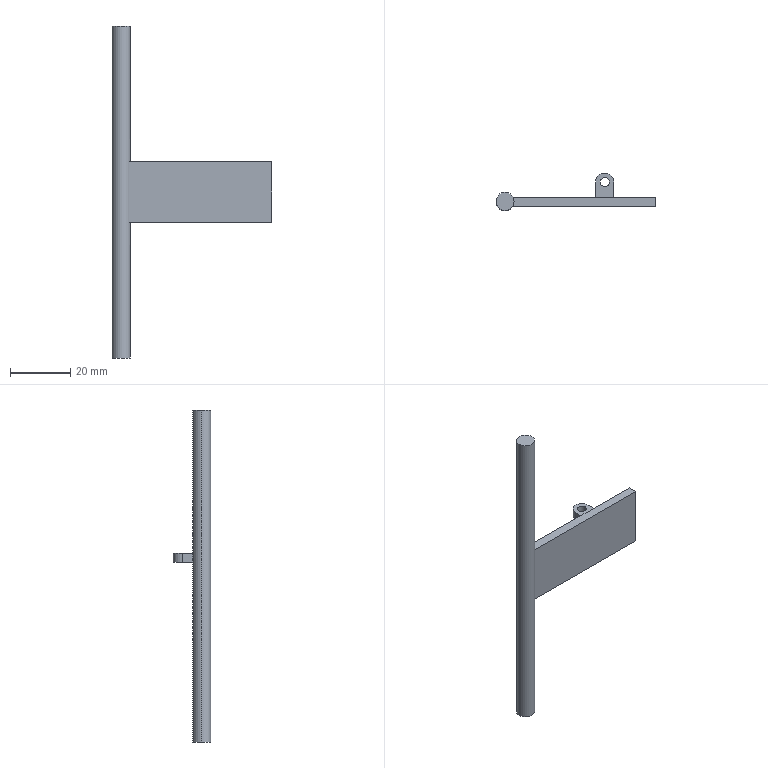Part | SolidWorks | features ICE 2, Extrusion 1 | 1 solid | 16 faces | box 53 x 12.5 x 110 mm | volume 6049 mm3 | plane 11 | cylinder 5 | commonest cylinder face diameters 6 x3 3 x2
STEP:
#1=CARTESIAN_POINT('',(31.5,6.5,4.5));
#2=VERTEX_POINT('',#1);
#3=CARTESIAN_POINT('',(34.5,6.5,4.5));
#4=VERTEX_POINT('',#3);
#5=CARTESIAN_POINT('',(33.,6.5,4.5));
#6=DIRECTION('',(0.,0.,1.));
#7=DIRECTION('',(1.,0.,0.));
#8=AXIS2_PLACEMENT_3D('',#5,#6,#7);
#9=CIRCLE('',#8,1.5);
#10=EDGE_CURVE('',#2,#4,#9,.T.);
#11=ORIENTED_EDGE('',*,*,#10,.F.);
#12=CARTESIAN_POINT('',(31.5,6.5,7.5));
#13=VERTEX_POINT('',#12);
#14=CARTESIAN_POINT('',(31.5,6.5,4.5));
#15=DIRECTION('',(0.,0.,1.));
#16=VECTOR('',#15,1000.);
#17=LINE('',#14,#16);
#18=EDGE_CURVE('',#2,#13,#17,.T.);
#19=ORIENTED_EDGE('',*,*,#18,.T.);
#20=CARTESIAN_POINT('',(34.5,6.5,7.5));
#21=VERTEX_POINT('',#20);
#22=CARTESIAN_POINT('',(33.,6.5,7.5));
#23=DIRECTION('',(0.,0.,1.));
#24=DIRECTION('',(1.,0.,0.));
#25=AXIS2_PLACEMENT_3D('',#22,#23,#24);
#26=CIRCLE('',#25,1.5);
#27=EDGE_CURVE('',#13,#21,#26,.T.);
#28=ORIENTED_EDGE('',*,*,#27,.T.);
#29=CARTESIAN_POINT('',(34.5,6.5,4.5));
#30=DIRECTION('',(0.,0.,1.));
#31=VECTOR('',#30,1000.);
#32=LINE('',#29,#31);
#33=EDGE_CURVE('',#4,#21,#32,.T.);
#34=ORIENTED_EDGE('',*,*,#33,.F.);
#35=EDGE_LOOP('',(#11,#19,#28,#34));
#36=FACE_OUTER_BOUND('',#35,.T.);
#37=CARTESIAN_POINT('',(33.,6.5,4.5));
#38=DIRECTION('',(0.,0.,1.));
#39=DIRECTION('',(1.,0.,0.));
#40=AXIS2_PLACEMENT_3D('',#37,#38,#39);
#41=CYLINDRICAL_SURFACE('',#40,1.5);
#42=ADVANCED_FACE('',(#36),#41,.F.);
#43=CARTESIAN_POINT('',(3.,0.,55.));
#44=VERTEX_POINT('',#43);
#45=CARTESIAN_POINT('',(-3.,0.,55.));
#46=VERTEX_POINT('',#45);
#47=CARTESIAN_POINT('',(0.,0.,55.));
#48=DIRECTION('',(0.,0.,1.));
#49=DIRECTION('',(1.,0.,0.));
#50=AXIS2_PLACEMENT_3D('',#47,#48,#49);
#51=CIRCLE('',#50,3.);
#52=EDGE_CURVE('',#44,#46,#51,.T.);
#53=ORIENTED_EDGE('',*,*,#52,.F.);
#54=CARTESIAN_POINT('',(3.,0.,10.));
#55=VERTEX_POINT('',#54);
#56=CARTESIAN_POINT('',(3.,0.,55.));
#57=DIRECTION('',(0.,0.,-1.));
#58=VECTOR('',#57,1000.);
#59=LINE('',#56,#58);
#60=EDGE_CURVE('',#44,#55,#59,.T.);
#61=ORIENTED_EDGE('',*,*,#60,.T.);
#62=CARTESIAN_POINT('',(2.598,1.5,10.));
#63=VERTEX_POINT('',#62);
#64=CARTESIAN_POINT('',(0.,0.,10.));
#65=DIRECTION('',(0.,0.,-1.));
#66=DIRECTION('',(-1.,0.,0.));
#67=AXIS2_PLACEMENT_3D('',#64,#65,#66);
#68=CIRCLE('',#67,3.);
#69=EDGE_CURVE('',#63,#55,#68,.T.);
#70=ORIENTED_EDGE('',*,*,#69,.F.);
#71=CARTESIAN_POINT('',(2.598,1.5,-10.));
#72=VERTEX_POINT('',#71);
#73=CARTESIAN_POINT('',(2.598,1.5,55.));
#74=DIRECTION('',(0.,0.,1.));
#75=VECTOR('',#74,1000.);
#76=LINE('',#73,#75);
#77=EDGE_CURVE('',#72,#63,#76,.T.);
#78=ORIENTED_EDGE('',*,*,#77,.F.);
#79=CARTESIAN_POINT('',(3.,0.,-10.));
#80=VERTEX_POINT('',#79);
#81=CARTESIAN_POINT('',(0.,0.,-10.));
#82=DIRECTION('',(0.,0.,-1.));
#83=DIRECTION('',(-1.,0.,0.));
#84=AXIS2_PLACEMENT_3D('',#81,#82,#83);
#85=CIRCLE('',#84,3.);
#86=EDGE_CURVE('',#72,#80,#85,.T.);
#87=ORIENTED_EDGE('',*,*,#86,.T.);
#88=CARTESIAN_POINT('',(3.,0.,-55.));
#89=VERTEX_POINT('',#88);
#90=CARTESIAN_POINT('',(3.,0.,55.));
#91=DIRECTION('',(0.,0.,-1.));
#92=VECTOR('',#91,1000.);
#93=LINE('',#90,#92);
#94=EDGE_CURVE('',#80,#89,#93,.T.);
#95=ORIENTED_EDGE('',*,*,#94,.T.);
#96=CARTESIAN_POINT('',(-3.,0.,-55.));
#97=VERTEX_POINT('',#96);
#98=CARTESIAN_POINT('',(0.,0.,-55.));
#99=DIRECTION('',(0.,0.,1.));
#100=DIRECTION('',(1.,0.,0.));
#101=AXIS2_PLACEMENT_3D('',#98,#99,#100);
#102=CIRCLE('',#101,3.);
#103=EDGE_CURVE('',#89,#97,#102,.T.);
#104=ORIENTED_EDGE('',*,*,#103,.T.);
#105=CARTESIAN_POINT('',(-3.,0.,55.));
#106=DIRECTION('',(0.,0.,-1.));
#107=VECTOR('',#106,1000.);
#108=LINE('',#105,#107);
#109=EDGE_CURVE('',#46,#97,#108,.T.);
#110=ORIENTED_EDGE('',*,*,#109,.F.);
#111=EDGE_LOOP('',(#53,#61,#70,#78,#87,#95,#104,#110));
#112=FACE_OUTER_BOUND('',#111,.T.);
#113=CARTESIAN_POINT('',(0.,0.,55.));
#114=DIRECTION('',(0.,0.,-1.));
#115=DIRECTION('',(-1.,0.,0.));
#116=AXIS2_PLACEMENT_3D('',#113,#114,#115);
#117=CYLINDRICAL_SURFACE('',#116,3.);
#118=ADVANCED_FACE('',(#112),#117,.T.);
#119=CARTESIAN_POINT('',(50.,1.5,-10.));
#120=VERTEX_POINT('',#119);
#121=CARTESIAN_POINT('',(50.,1.5,-10.));
#122=DIRECTION('',(-1.,0.,0.));
#123=VECTOR('',#122,1000.);
#124=LINE('',#121,#123);
#125=EDGE_CURVE('',#120,#72,#124,.T.);
#126=ORIENTED_EDGE('',*,*,#125,.T.);
#127=ORIENTED_EDGE('',*,*,#77,.T.);
#128=CARTESIAN_POINT('',(50.,1.5,10.));
#129=VERTEX_POINT('',#128);
#130=CARTESIAN_POINT('',(50.,1.5,10.));
#131=DIRECTION('',(-1.,0.,0.));
#132=VECTOR('',#131,1000.);
#133=LINE('',#130,#132);
#134=EDGE_CURVE('',#129,#63,#133,.T.);
#135=ORIENTED_EDGE('',*,*,#134,.F.);
#136=CARTESIAN_POINT('',(50.,1.5,10.));
#137=DIRECTION('',(0.,0.,-1.));
#138=VECTOR('',#137,1000.);
#139=LINE('',#136,#138);
#140=EDGE_CURVE('',#129,#120,#139,.T.);
#141=ORIENTED_EDGE('',*,*,#140,.T.);
#142=EDGE_LOOP('',(#126,#127,#135,#141));
#143=FACE_OUTER_BOUND('',#142,.T.);
#144=CARTESIAN_POINT('',(30.,1.5,4.5));
#145=VERTEX_POINT('',#144);
#146=CARTESIAN_POINT('',(36.,1.5,4.5));
#147=VERTEX_POINT('',#146);
#148=CARTESIAN_POINT('',(0.,1.5,4.5));
#149=DIRECTION('',(1.,0.,0.));
#150=VECTOR('',#149,1000.);
#151=LINE('',#148,#150);
#152=EDGE_CURVE('',#145,#147,#151,.T.);
#153=ORIENTED_EDGE('',*,*,#152,.T.);
#154=CARTESIAN_POINT('',(36.,1.5,7.5));
#155=VERTEX_POINT('',#154);
#156=CARTESIAN_POINT('',(36.,1.5,4.5));
#157=DIRECTION('',(0.,0.,1.));
#158=VECTOR('',#157,1000.);
#159=LINE('',#156,#158);
#160=EDGE_CURVE('',#147,#155,#159,.T.);
#161=ORIENTED_EDGE('',*,*,#160,.T.);
#162=CARTESIAN_POINT('',(30.,1.5,7.5));
#163=VERTEX_POINT('',#162);
#164=CARTESIAN_POINT('',(0.,1.5,7.5));
#165=DIRECTION('',(1.,0.,0.));
#166=VECTOR('',#165,1000.);
#167=LINE('',#164,#166);
#168=EDGE_CURVE('',#163,#155,#167,.T.);
#169=ORIENTED_EDGE('',*,*,#168,.F.);
#170=CARTESIAN_POINT('',(30.,1.5,4.5));
#171=DIRECTION('',(0.,0.,1.));
#172=VECTOR('',#171,1000.);
#173=LINE('',#170,#172);
#174=EDGE_CURVE('',#145,#163,#173,.T.);
#175=ORIENTED_EDGE('',*,*,#174,.F.);
#176=EDGE_LOOP('',(#153,#161,#169,#175));
#177=FACE_BOUND('',#176,.T.);
#178=CARTESIAN_POINT('',(50.,1.5,10.));
#179=DIRECTION('',(0.,-1.,0.));
#180=DIRECTION('',(0.,0.,-1.));
#181=AXIS2_PLACEMENT_3D('',#178,#179,#180);
#182=PLANE('',#181);
#183=ADVANCED_FACE('',(#143,#177),#182,.F.);
#184=ORIENTED_EDGE('',*,*,#60,.F.);
#185=CARTESIAN_POINT('',(0.,0.,55.));
#186=DIRECTION('',(0.,0.,1.));
#187=DIRECTION('',(1.,0.,0.));
#188=AXIS2_PLACEMENT_3D('',#185,#186,#187);
#189=CIRCLE('',#188,3.);
#190=EDGE_CURVE('',#46,#44,#189,.T.);
#191=ORIENTED_EDGE('',*,*,#190,.F.);
#192=ORIENTED_EDGE('',*,*,#109,.T.);
#193=CARTESIAN_POINT('',(0.,0.,-55.));
#194=DIRECTION('',(0.,0.,1.));
#195=DIRECTION('',(1.,0.,0.));
#196=AXIS2_PLACEMENT_3D('',#193,#194,#195);
#197=CIRCLE('',#196,3.);
#198=EDGE_CURVE('',#97,#89,#197,.T.);
#199=ORIENTED_EDGE('',*,*,#198,.T.);
#200=ORIENTED_EDGE('',*,*,#94,.F.);
#201=CARTESIAN_POINT('',(2.598,-1.5,-10.));
#202=VERTEX_POINT('',#201);
#203=CARTESIAN_POINT('',(0.,0.,-10.));
#204=DIRECTION('',(0.,0.,-1.));
#205=DIRECTION('',(-1.,0.,0.));
#206=AXIS2_PLACEMENT_3D('',#203,#204,#205);
#207=CIRCLE('',#206,3.);
#208=EDGE_CURVE('',#80,#202,#207,.T.);
#209=ORIENTED_EDGE('',*,*,#208,.T.);
#210=CARTESIAN_POINT('',(2.598,-1.5,10.));
#211=VERTEX_POINT('',#210);
#212=CARTESIAN_POINT('',(2.598,-1.5,55.));
#213=DIRECTION('',(0.,0.,-1.));
#214=VECTOR('',#213,1000.);
#215=LINE('',#212,#214);
#216=EDGE_CURVE('',#211,#202,#215,.T.);
#217=ORIENTED_EDGE('',*,*,#216,.F.);
#218=CARTESIAN_POINT('',(0.,0.,10.));
#219=DIRECTION('',(0.,0.,-1.));
#220=DIRECTION('',(-1.,0.,0.));
#221=AXIS2_PLACEMENT_3D('',#218,#219,#220);
#222=CIRCLE('',#221,3.);
#223=EDGE_CURVE('',#55,#211,#222,.T.);
#224=ORIENTED_EDGE('',*,*,#223,.F.);
#225=EDGE_LOOP('',(#184,#191,#192,#199,#200,#209,#217,#224));
#226=FACE_OUTER_BOUND('',#225,.T.);
#227=CARTESIAN_POINT('',(0.,0.,55.));
#228=DIRECTION('',(0.,0.,-1.));
#229=DIRECTION('',(-1.,0.,0.));
#230=AXIS2_PLACEMENT_3D('',#227,#228,#229);
#231=CYLINDRICAL_SURFACE('',#230,3.);
#232=ADVANCED_FACE('',(#226),#231,.T.);
#233=ORIENTED_EDGE('',*,*,#190,.T.);
#234=ORIENTED_EDGE('',*,*,#52,.T.);
#235=EDGE_LOOP('',(#233,#234));
#236=FACE_OUTER_BOUND('',#235,.T.);
#237=CARTESIAN_POINT('',(0.,0.,55.));
#238=DIRECTION('',(0.,0.,1.));
#239=DIRECTION('',(1.,0.,0.));
#240=AXIS2_PLACEMENT_3D('',#237,#238,#239);
#241=PLANE('',#240);
#242=ADVANCED_FACE('',(#236),#241,.T.);
#243=ORIENTED_EDGE('',*,*,#198,.F.);
#244=ORIENTED_EDGE('',*,*,#103,.F.);
#245=EDGE_LOOP('',(#243,#244));
#246=FACE_OUTER_BOUND('',#245,.T.);
#247=CARTESIAN_POINT('',(0.,0.,-55.));
#248=DIRECTION('',(0.,0.,1.));
#249=DIRECTION('',(1.,0.,0.));
#250=AXIS2_PLACEMENT_3D('',#247,#248,#249);
#251=PLANE('',#250);
#252=ADVANCED_FACE('',(#246),#251,.F.);
#253=CARTESIAN_POINT('',(50.,-1.5,10.));
#254=VERTEX_POINT('',#253);
#255=CARTESIAN_POINT('',(50.,-1.5,10.));
#256=DIRECTION('',(1.,0.,0.));
#257=VECTOR('',#256,1000.);
#258=LINE('',#255,#257);
#259=EDGE_CURVE('',#211,#254,#258,.T.);
#260=ORIENTED_EDGE('',*,*,#259,.F.);
#261=ORIENTED_EDGE('',*,*,#216,.T.);
#262=CARTESIAN_POINT('',(50.,-1.5,-10.));
#263=VERTEX_POINT('',#262);
#264=CARTESIAN_POINT('',(50.,-1.5,-10.));
#265=DIRECTION('',(1.,0.,0.));
#266=VECTOR('',#265,1000.);
#267=LINE('',#264,#266);
#268=EDGE_CURVE('',#202,#263,#267,.T.);
#269=ORIENTED_EDGE('',*,*,#268,.T.);
#270=CARTESIAN_POINT('',(50.,-1.5,10.));
#271=DIRECTION('',(0.,0.,-1.));
#272=VECTOR('',#271,1000.);
#273=LINE('',#270,#272);
#274=EDGE_CURVE('',#254,#263,#273,.T.);
#275=ORIENTED_EDGE('',*,*,#274,.F.);
#276=EDGE_LOOP('',(#260,#261,#269,#275));
#277=FACE_OUTER_BOUND('',#276,.T.);
#278=CARTESIAN_POINT('',(50.,-1.5,10.));
#279=DIRECTION('',(0.,1.,0.));
#280=DIRECTION('',(0.,0.,1.));
#281=AXIS2_PLACEMENT_3D('',#278,#279,#280);
#282=PLANE('',#281);
#283=ADVANCED_FACE('',(#277),#282,.F.);
#284=CARTESIAN_POINT('',(50.,1.5,-10.));
#285=DIRECTION('',(0.,1.,0.));
#286=VECTOR('',#285,1000.);
#287=LINE('',#284,#286);
#288=EDGE_CURVE('',#263,#120,#287,.T.);
#289=ORIENTED_EDGE('',*,*,#288,.T.);
#290=ORIENTED_EDGE('',*,*,#140,.F.);
#291=CARTESIAN_POINT('',(50.,1.5,10.));
#292=DIRECTION('',(0.,1.,0.));
#293=VECTOR('',#292,1000.);
#294=LINE('',#291,#293);
#295=EDGE_CURVE('',#254,#129,#294,.T.);
#296=ORIENTED_EDGE('',*,*,#295,.F.);
#297=ORIENTED_EDGE('',*,*,#274,.T.);
#298=EDGE_LOOP('',(#289,#290,#296,#297));
#299=FACE_OUTER_BOUND('',#298,.T.);
#300=CARTESIAN_POINT('',(50.,1.5,10.));
#301=DIRECTION('',(-1.,0.,0.));
#302=DIRECTION('',(0.,0.,1.));
#303=AXIS2_PLACEMENT_3D('',#300,#301,#302);
#304=PLANE('',#303);
#305=ADVANCED_FACE('',(#299),#304,.F.);
#306=ORIENTED_EDGE('',*,*,#134,.T.);
#307=ORIENTED_EDGE('',*,*,#69,.T.);
#308=ORIENTED_EDGE('',*,*,#223,.T.);
#309=ORIENTED_EDGE('',*,*,#259,.T.);
#310=ORIENTED_EDGE('',*,*,#295,.T.);
#311=EDGE_LOOP('',(#306,#307,#308,#309,#310));
#312=FACE_OUTER_BOUND('',#311,.T.);
#313=CARTESIAN_POINT('',(0.,0.,10.));
#314=DIRECTION('',(0.,0.,-1.));
#315=DIRECTION('',(-1.,0.,0.));
#316=AXIS2_PLACEMENT_3D('',#313,#314,#315);
#317=PLANE('',#316);
#318=ADVANCED_FACE('',(#312),#317,.F.);
#319=ORIENTED_EDGE('',*,*,#86,.F.);
#320=ORIENTED_EDGE('',*,*,#125,.F.);
#321=ORIENTED_EDGE('',*,*,#288,.F.);
#322=ORIENTED_EDGE('',*,*,#268,.F.);
#323=ORIENTED_EDGE('',*,*,#208,.F.);
#324=EDGE_LOOP('',(#319,#320,#321,#322,#323));
#325=FACE_OUTER_BOUND('',#324,.T.);
#326=CARTESIAN_POINT('',(0.,0.,-10.));
#327=DIRECTION('',(0.,0.,-1.));
#328=DIRECTION('',(-1.,0.,0.));
#329=AXIS2_PLACEMENT_3D('',#326,#327,#328);
#330=PLANE('',#329);
#331=ADVANCED_FACE('',(#325),#330,.T.);
#332=CARTESIAN_POINT('',(36.,6.5,7.5));
#333=VERTEX_POINT('',#332);
#334=CARTESIAN_POINT('',(30.,6.5,7.5));
#335=VERTEX_POINT('',#334);
#336=CARTESIAN_POINT('',(33.,6.5,7.5));
#337=DIRECTION('',(0.,0.,1.));
#338=DIRECTION('',(1.,0.,0.));
#339=AXIS2_PLACEMENT_3D('',#336,#337,#338);
#340=CIRCLE('',#339,3.);
#341=EDGE_CURVE('',#333,#335,#340,.T.);
#342=ORIENTED_EDGE('',*,*,#341,.F.);
#343=CARTESIAN_POINT('',(36.,6.5,4.5));
#344=VERTEX_POINT('',#343);
#345=CARTESIAN_POINT('',(36.,6.5,4.5));
#346=DIRECTION('',(0.,0.,1.));
#347=VECTOR('',#346,1000.);
#348=LINE('',#345,#347);
#349=EDGE_CURVE('',#344,#333,#348,.T.);
#350=ORIENTED_EDGE('',*,*,#349,.F.);
#351=CARTESIAN_POINT('',(30.,6.5,4.5));
#352=VERTEX_POINT('',#351);
#353=CARTESIAN_POINT('',(33.,6.5,4.5));
#354=DIRECTION('',(0.,0.,1.));
#355=DIRECTION('',(1.,0.,0.));
#356=AXIS2_PLACEMENT_3D('',#353,#354,#355);
#357=CIRCLE('',#356,3.);
#358=EDGE_CURVE('',#344,#352,#357,.T.);
#359=ORIENTED_EDGE('',*,*,#358,.T.);
#360=CARTESIAN_POINT('',(30.,6.5,4.5));
#361=DIRECTION('',(0.,0.,1.));
#362=VECTOR('',#361,1000.);
#363=LINE('',#360,#362);
#364=EDGE_CURVE('',#352,#335,#363,.T.);
#365=ORIENTED_EDGE('',*,*,#364,.T.);
#366=EDGE_LOOP('',(#342,#350,#359,#365));
#367=FACE_OUTER_BOUND('',#366,.T.);
#368=CARTESIAN_POINT('',(33.,6.5,4.5));
#369=DIRECTION('',(0.,0.,1.));
#370=DIRECTION('',(1.,0.,0.));
#371=AXIS2_PLACEMENT_3D('',#368,#369,#370);
#372=CYLINDRICAL_SURFACE('',#371,3.);
#373=ADVANCED_FACE('',(#367),#372,.T.);
#374=CARTESIAN_POINT('',(36.,0.,7.5));
#375=DIRECTION('',(0.,1.,0.));
#376=VECTOR('',#375,1000.);
#377=LINE('',#374,#376);
#378=EDGE_CURVE('',#155,#333,#377,.T.);
#379=ORIENTED_EDGE('',*,*,#378,.F.);
#380=ORIENTED_EDGE('',*,*,#160,.F.);
#381=CARTESIAN_POINT('',(36.,0.,4.5));
#382=DIRECTION('',(0.,1.,0.));
#383=VECTOR('',#382,1000.);
#384=LINE('',#381,#383);
#385=EDGE_CURVE('',#147,#344,#384,.T.);
#386=ORIENTED_EDGE('',*,*,#385,.T.);
#387=ORIENTED_EDGE('',*,*,#349,.T.);
#388=EDGE_LOOP('',(#379,#380,#386,#387));
#389=FACE_OUTER_BOUND('',#388,.T.);
#390=CARTESIAN_POINT('',(36.,0.,4.5));
#391=DIRECTION('',(1.,0.,0.));
#392=DIRECTION('',(0.,0.,-1.));
#393=AXIS2_PLACEMENT_3D('',#390,#391,#392);
#394=PLANE('',#393);
#395=ADVANCED_FACE('',(#389),#394,.T.);
#396=ORIENTED_EDGE('',*,*,#18,.F.);
#397=CARTESIAN_POINT('',(33.,6.5,4.5));
#398=DIRECTION('',(0.,0.,1.));
#399=DIRECTION('',(1.,0.,0.));
#400=AXIS2_PLACEMENT_3D('',#397,#398,#399);
#401=CIRCLE('',#400,1.5);
#402=EDGE_CURVE('',#4,#2,#401,.T.);
#403=ORIENTED_EDGE('',*,*,#402,.F.);
#404=ORIENTED_EDGE('',*,*,#33,.T.);
#405=CARTESIAN_POINT('',(33.,6.5,7.5));
#406=DIRECTION('',(0.,0.,1.));
#407=DIRECTION('',(1.,0.,0.));
#408=AXIS2_PLACEMENT_3D('',#405,#406,#407);
#409=CIRCLE('',#408,1.5);
#410=EDGE_CURVE('',#21,#13,#409,.T.);
#411=ORIENTED_EDGE('',*,*,#410,.T.);
#412=EDGE_LOOP('',(#396,#403,#404,#411));
#413=FACE_OUTER_BOUND('',#412,.T.);
#414=CARTESIAN_POINT('',(33.,6.5,4.5));
#415=DIRECTION('',(0.,0.,1.));
#416=DIRECTION('',(1.,0.,0.));
#417=AXIS2_PLACEMENT_3D('',#414,#415,#416);
#418=CYLINDRICAL_SURFACE('',#417,1.5);
#419=ADVANCED_FACE('',(#413),#418,.F.);
#420=CARTESIAN_POINT('',(30.,0.,7.5));
#421=DIRECTION('',(0.,-1.,0.));
#422=VECTOR('',#421,1000.);
#423=LINE('',#420,#422);
#424=EDGE_CURVE('',#335,#163,#423,.T.);
#425=ORIENTED_EDGE('',*,*,#424,.F.);
#426=ORIENTED_EDGE('',*,*,#364,.F.);
#427=CARTESIAN_POINT('',(30.,0.,4.5));
#428=DIRECTION('',(0.,-1.,0.));
#429=VECTOR('',#428,1000.);
#430=LINE('',#427,#429);
#431=EDGE_CURVE('',#352,#145,#430,.T.);
#432=ORIENTED_EDGE('',*,*,#431,.T.);
#433=ORIENTED_EDGE('',*,*,#174,.T.);
#434=EDGE_LOOP('',(#425,#426,#432,#433));
#435=FACE_OUTER_BOUND('',#434,.T.);
#436=CARTESIAN_POINT('',(30.,0.,4.5));
#437=DIRECTION('',(-1.,0.,0.));
#438=DIRECTION('',(0.,0.,1.));
#439=AXIS2_PLACEMENT_3D('',#436,#437,#438);
#440=PLANE('',#439);
#441=ADVANCED_FACE('',(#435),#440,.T.);
#442=ORIENTED_EDGE('',*,*,#402,.T.);
#443=ORIENTED_EDGE('',*,*,#10,.T.);
#444=EDGE_LOOP('',(#442,#443));
#445=FACE_BOUND('',#444,.T.);
#446=ORIENTED_EDGE('',*,*,#358,.F.);
#447=ORIENTED_EDGE('',*,*,#385,.F.);
#448=ORIENTED_EDGE('',*,*,#152,.F.);
#449=ORIENTED_EDGE('',*,*,#431,.F.);
#450=EDGE_LOOP('',(#446,#447,#448,#449));
#451=FACE_OUTER_BOUND('',#450,.T.);
#452=CARTESIAN_POINT('',(0.,0.,4.5));
#453=DIRECTION('',(0.,0.,1.));
#454=DIRECTION('',(1.,0.,0.));
#455=AXIS2_PLACEMENT_3D('',#452,#453,#454);
#456=PLANE('',#455);
#457=ADVANCED_FACE('',(#445,#451),#456,.F.);
#458=ORIENTED_EDGE('',*,*,#410,.F.);
#459=ORIENTED_EDGE('',*,*,#27,.F.);
#460=EDGE_LOOP('',(#458,#459));
#461=FACE_BOUND('',#460,.T.);
#462=ORIENTED_EDGE('',*,*,#341,.T.);
#463=ORIENTED_EDGE('',*,*,#424,.T.);
#464=ORIENTED_EDGE('',*,*,#168,.T.);
#465=ORIENTED_EDGE('',*,*,#378,.T.);
#466=EDGE_LOOP('',(#462,#463,#464,#465));
#467=FACE_OUTER_BOUND('',#466,.T.);
#468=CARTESIAN_POINT('',(0.,0.,7.5));
#469=DIRECTION('',(0.,0.,1.));
#470=DIRECTION('',(1.,0.,0.));
#471=AXIS2_PLACEMENT_3D('',#468,#469,#470);
#472=PLANE('',#471);
#473=ADVANCED_FACE('',(#461,#467),#472,.T.);
#474=CLOSED_SHELL('',(#42,#118,#183,#232,#242,#252,#283,#305,#318,#331,#373,#395,#419,#441,#457,#473));
#475=MANIFOLD_SOLID_BREP('',#474);
#476=CARTESIAN_POINT('',(0.,0.,0.));
#477=DIRECTION('',(0.,0.,1.));
#478=DIRECTION('',(1.,0.,0.));
#479=AXIS2_PLACEMENT_3D('',#476,#477,#478);
#480=(LENGTH_UNIT()NAMED_UNIT(*)SI_UNIT(.MILLI.,.METRE.));
#481=UNCERTAINTY_MEASURE_WITH_UNIT(LENGTH_MEASURE(0.00001),#480,'','');
#482=(NAMED_UNIT(*)PLANE_ANGLE_UNIT()SI_UNIT($,.RADIAN.));
#483=(NAMED_UNIT(*)SI_UNIT($,.STERADIAN.)SOLID_ANGLE_UNIT());
#484=(GEOMETRIC_REPRESENTATION_CONTEXT(3)GLOBAL_UNCERTAINTY_ASSIGNED_CONTEXT((#481))GLOBAL_UNIT_ASSIGNED_CONTEXT((#480,#482,#483))REPRESENTATION_CONTEXT('',''));
#485=ADVANCED_BREP_SHAPE_REPRESENTATION('',(#475,#479),#484);